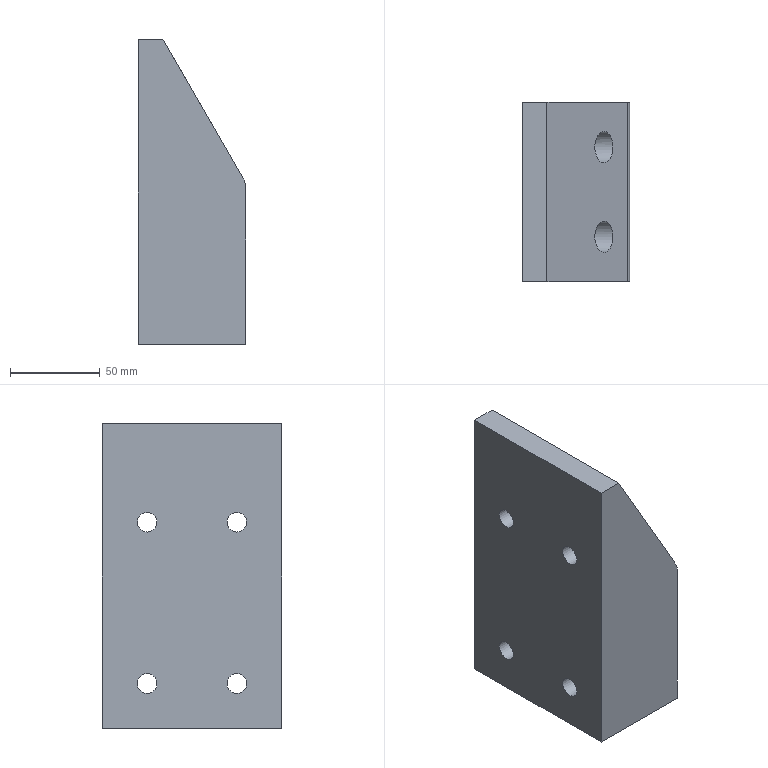Part | NX | features MAIN_BODY 2 | 1 solid | 20 faces | box 60 x 100 x 170 mm | volume 796043 mm3 | plane 11 | cylinder 9 | commonest cylinder face diameters 11 x4 17.5 x4 20 x1
STEP:
#1=CARTESIAN_POINT('',(1053.66,140.,-57.679));
#2=VERTEX_POINT('',#1);
#3=CARTESIAN_POINT('',(1008.812,140.,20.));
#4=VERTEX_POINT('',#3);
#5=CARTESIAN_POINT('',(1094.748,140.,-128.846));
#6=DIRECTION('',(-0.5,0.,0.866));
#7=VECTOR('',#6,1000.);
#8=LINE('',#5,#7);
#9=EDGE_CURVE('',#2,#4,#8,.T.);
#10=ORIENTED_EDGE('',*,*,#9,.T.);
#11=CARTESIAN_POINT('',(995.,140.,20.));
#12=VERTEX_POINT('',#11);
#13=CARTESIAN_POINT('',(850.,140.,20.));
#14=DIRECTION('',(-1.,0.,0.));
#15=VECTOR('',#14,1000.);
#16=LINE('',#13,#15);
#17=EDGE_CURVE('',#4,#12,#16,.T.);
#18=ORIENTED_EDGE('',*,*,#17,.T.);
#19=CARTESIAN_POINT('',(995.,140.,-150.));
#20=VERTEX_POINT('',#19);
#21=CARTESIAN_POINT('',(995.,140.,-335.));
#22=DIRECTION('',(0.,0.,1.));
#23=VECTOR('',#22,1000.);
#24=LINE('',#21,#23);
#25=EDGE_CURVE('',#20,#12,#24,.T.);
#26=ORIENTED_EDGE('',*,*,#25,.F.);
#27=CARTESIAN_POINT('',(1055.,140.,-150.));
#28=VERTEX_POINT('',#27);
#29=CARTESIAN_POINT('',(906.301,140.,-150.));
#30=DIRECTION('',(1.,0.,0.));
#31=VECTOR('',#30,1000.);
#32=LINE('',#29,#31);
#33=EDGE_CURVE('',#20,#28,#32,.T.);
#34=ORIENTED_EDGE('',*,*,#33,.T.);
#35=CARTESIAN_POINT('',(1055.,140.,-62.679));
#36=VERTEX_POINT('',#35);
#37=CARTESIAN_POINT('',(1055.,140.,-335.));
#38=DIRECTION('',(0.,0.,-1.));
#39=VECTOR('',#38,1000.);
#40=LINE('',#37,#39);
#41=EDGE_CURVE('',#36,#28,#40,.T.);
#42=ORIENTED_EDGE('',*,*,#41,.F.);
#43=CARTESIAN_POINT('',(1045.,140.,-62.679));
#44=DIRECTION('',(0.,-1.,0.));
#45=DIRECTION('',(1.,0.,0.));
#46=AXIS2_PLACEMENT_3D('',#43,#44,#45);
#47=CIRCLE('',#46,10.);
#48=EDGE_CURVE('',#2,#36,#47,.F.);
#49=ORIENTED_EDGE('',*,*,#48,.F.);
#50=EDGE_LOOP('',(#10,#18,#26,#34,#42,#49));
#51=FACE_BOUND('',#50,.T.);
#52=CARTESIAN_POINT('',(865.,140.,-335.));
#53=DIRECTION('',(0.,1.,0.));
#54=DIRECTION('',(0.,0.,1.));
#55=AXIS2_PLACEMENT_3D('',#52,#53,#54);
#56=PLANE('',#55);
#57=ADVANCED_FACE('',(#51),#56,.F.);
#58=CARTESIAN_POINT('',(1055.,240.,-150.));
#59=VERTEX_POINT('',#58);
#60=CARTESIAN_POINT('',(1055.,240.,-62.679));
#61=VERTEX_POINT('',#60);
#62=CARTESIAN_POINT('',(1055.,240.,-335.));
#63=DIRECTION('',(0.,0.,-1.));
#64=VECTOR('',#63,1000.);
#65=LINE('',#62,#64);
#66=EDGE_CURVE('',#59,#61,#65,.F.);
#67=ORIENTED_EDGE('',*,*,#66,.F.);
#68=CARTESIAN_POINT('',(995.,240.,-150.));
#69=VERTEX_POINT('',#68);
#70=CARTESIAN_POINT('',(906.301,240.,-150.));
#71=DIRECTION('',(1.,0.,0.));
#72=VECTOR('',#71,1000.);
#73=LINE('',#70,#72);
#74=EDGE_CURVE('',#59,#69,#73,.F.);
#75=ORIENTED_EDGE('',*,*,#74,.T.);
#76=CARTESIAN_POINT('',(995.,240.,20.));
#77=VERTEX_POINT('',#76);
#78=CARTESIAN_POINT('',(995.,240.,-335.));
#79=DIRECTION('',(0.,0.,-1.));
#80=VECTOR('',#79,1000.);
#81=LINE('',#78,#80);
#82=EDGE_CURVE('',#69,#77,#81,.F.);
#83=ORIENTED_EDGE('',*,*,#82,.T.);
#84=CARTESIAN_POINT('',(1008.812,240.,20.));
#85=VERTEX_POINT('',#84);
#86=CARTESIAN_POINT('',(850.,240.,20.));
#87=DIRECTION('',(-1.,0.,0.));
#88=VECTOR('',#87,1000.);
#89=LINE('',#86,#88);
#90=EDGE_CURVE('',#77,#85,#89,.F.);
#91=ORIENTED_EDGE('',*,*,#90,.T.);
#92=CARTESIAN_POINT('',(1053.66,240.,-57.679));
#93=VERTEX_POINT('',#92);
#94=CARTESIAN_POINT('',(1094.748,240.,-128.846));
#95=DIRECTION('',(-0.5,0.,0.866));
#96=VECTOR('',#95,1000.);
#97=LINE('',#94,#96);
#98=EDGE_CURVE('',#93,#85,#97,.T.);
#99=ORIENTED_EDGE('',*,*,#98,.F.);
#100=CARTESIAN_POINT('',(1045.,240.,-62.679));
#101=DIRECTION('',(0.,-1.,0.));
#102=DIRECTION('',(1.,0.,0.));
#103=AXIS2_PLACEMENT_3D('',#100,#101,#102);
#104=CIRCLE('',#103,10.);
#105=EDGE_CURVE('',#61,#93,#104,.T.);
#106=ORIENTED_EDGE('',*,*,#105,.F.);
#107=EDGE_LOOP('',(#67,#75,#83,#91,#99,#106));
#108=FACE_BOUND('',#107,.T.);
#109=CARTESIAN_POINT('',(865.,240.,-335.));
#110=DIRECTION('',(0.,1.,0.));
#111=DIRECTION('',(0.,0.,1.));
#112=AXIS2_PLACEMENT_3D('',#109,#110,#111);
#113=PLANE('',#112);
#114=ADVANCED_FACE('',(#108),#113,.T.);
#115=CARTESIAN_POINT('',(1055.,223.75,-125.));
#116=VERTEX_POINT('',#115);
#117=CARTESIAN_POINT('',(1055.,215.,-125.));
#118=DIRECTION('',(-1.,0.,0.));
#119=DIRECTION('',(0.,1.,0.));
#120=AXIS2_PLACEMENT_3D('',#117,#118,#119);
#121=CIRCLE('',#120,8.75);
#122=EDGE_CURVE('',#116,#116,#121,.T.);
#123=ORIENTED_EDGE('',*,*,#122,.T.);
#124=EDGE_LOOP('',(#123));
#125=FACE_BOUND('',#124,.T.);
#126=CARTESIAN_POINT('',(1055.,173.75,-125.));
#127=VERTEX_POINT('',#126);
#128=CARTESIAN_POINT('',(1055.,165.,-125.));
#129=DIRECTION('',(-1.,0.,0.));
#130=DIRECTION('',(0.,1.,0.));
#131=AXIS2_PLACEMENT_3D('',#128,#129,#130);
#132=CIRCLE('',#131,8.75);
#133=EDGE_CURVE('',#127,#127,#132,.T.);
#134=ORIENTED_EDGE('',*,*,#133,.T.);
#135=EDGE_LOOP('',(#134));
#136=FACE_BOUND('',#135,.T.);
#137=ORIENTED_EDGE('',*,*,#41,.T.);
#138=CARTESIAN_POINT('',(1055.,114.375,-150.));
#139=DIRECTION('',(0.,1.,0.));
#140=VECTOR('',#139,1000.);
#141=LINE('',#138,#140);
#142=EDGE_CURVE('',#28,#59,#141,.T.);
#143=ORIENTED_EDGE('',*,*,#142,.T.);
#144=ORIENTED_EDGE('',*,*,#66,.T.);
#145=CARTESIAN_POINT('',(1055.,230.,-62.679));
#146=DIRECTION('',(0.,-1.,0.));
#147=VECTOR('',#146,1000.);
#148=LINE('',#145,#147);
#149=EDGE_CURVE('',#36,#61,#148,.F.);
#150=ORIENTED_EDGE('',*,*,#149,.F.);
#151=EDGE_LOOP('',(#137,#143,#144,#150));
#152=FACE_BOUND('',#151,.T.);
#153=CARTESIAN_POINT('',(1055.,190.,-105.));
#154=DIRECTION('',(-1.,0.,0.));
#155=DIRECTION('',(0.,-1.,0.));
#156=AXIS2_PLACEMENT_3D('',#153,#154,#155);
#157=PLANE('',#156);
#158=ADVANCED_FACE('',(#125,#136,#152),#157,.F.);
#159=CARTESIAN_POINT('',(1015.,165.,-26.25));
#160=VERTEX_POINT('',#159);
#161=CARTESIAN_POINT('',(1015.,165.,-35.));
#162=DIRECTION('',(-1.,0.,0.));
#163=DIRECTION('',(0.,0.,1.));
#164=AXIS2_PLACEMENT_3D('',#161,#162,#163);
#165=CIRCLE('',#164,8.75);
#166=EDGE_CURVE('',#160,#160,#165,.T.);
#167=ORIENTED_EDGE('',*,*,#166,.T.);
#168=EDGE_LOOP('',(#167));
#169=FACE_BOUND('',#168,.T.);
#170=CARTESIAN_POINT('',(1045.618,165.,-43.75));
#171=VERTEX_POINT('',#170);
#172=CARTESIAN_POINT('',(1040.566,165.,-35.));
#173=DIRECTION('',(-0.866,0.,-0.5));
#174=DIRECTION('',(0.5,0.,-0.866));
#175=AXIS2_PLACEMENT_3D('',#172,#173,#174);
#176=ELLIPSE('',#175,10.104,8.75);
#177=EDGE_CURVE('',#171,#171,#176,.F.);
#178=ORIENTED_EDGE('',*,*,#177,.T.);
#179=EDGE_LOOP('',(#178));
#180=FACE_BOUND('',#179,.T.);
#181=CARTESIAN_POINT('',(1020.,165.,-35.));
#182=DIRECTION('',(1.,0.,0.));
#183=DIRECTION('',(0.,0.,1.));
#184=AXIS2_PLACEMENT_3D('',#181,#182,#183);
#185=CYLINDRICAL_SURFACE('',#184,8.75);
#186=ADVANCED_FACE('',(#169,#180),#185,.F.);
#187=CARTESIAN_POINT('',(1015.,215.,-26.25));
#188=VERTEX_POINT('',#187);
#189=CARTESIAN_POINT('',(1015.,215.,-35.));
#190=DIRECTION('',(-1.,0.,0.));
#191=DIRECTION('',(0.,0.,1.));
#192=AXIS2_PLACEMENT_3D('',#189,#190,#191);
#193=CIRCLE('',#192,8.75);
#194=EDGE_CURVE('',#188,#188,#193,.T.);
#195=ORIENTED_EDGE('',*,*,#194,.T.);
#196=EDGE_LOOP('',(#195));
#197=FACE_BOUND('',#196,.T.);
#198=CARTESIAN_POINT('',(1045.618,215.,-43.75));
#199=VERTEX_POINT('',#198);
#200=CARTESIAN_POINT('',(1040.566,215.,-35.));
#201=DIRECTION('',(-0.866,0.,-0.5));
#202=DIRECTION('',(0.5,0.,-0.866));
#203=AXIS2_PLACEMENT_3D('',#200,#201,#202);
#204=ELLIPSE('',#203,10.104,8.75);
#205=EDGE_CURVE('',#199,#199,#204,.F.);
#206=ORIENTED_EDGE('',*,*,#205,.T.);
#207=EDGE_LOOP('',(#206));
#208=FACE_BOUND('',#207,.T.);
#209=CARTESIAN_POINT('',(1020.,215.,-35.));
#210=DIRECTION('',(1.,0.,0.));
#211=DIRECTION('',(0.,0.,1.));
#212=AXIS2_PLACEMENT_3D('',#209,#210,#211);
#213=CYLINDRICAL_SURFACE('',#212,8.75);
#214=ADVANCED_FACE('',(#197,#208),#213,.F.);
#215=CARTESIAN_POINT('',(995.,165.,-29.5));
#216=VERTEX_POINT('',#215);
#217=CARTESIAN_POINT('',(995.,165.,-35.));
#218=DIRECTION('',(-1.,0.,0.));
#219=DIRECTION('',(0.,0.,1.));
#220=AXIS2_PLACEMENT_3D('',#217,#218,#219);
#221=CIRCLE('',#220,5.5);
#222=EDGE_CURVE('',#216,#216,#221,.F.);
#223=ORIENTED_EDGE('',*,*,#222,.T.);
#224=EDGE_LOOP('',(#223));
#225=FACE_BOUND('',#224,.T.);
#226=CARTESIAN_POINT('',(995.,165.,-119.5));
#227=VERTEX_POINT('',#226);
#228=CARTESIAN_POINT('',(995.,165.,-125.));
#229=DIRECTION('',(-1.,0.,0.));
#230=DIRECTION('',(0.,0.,1.));
#231=AXIS2_PLACEMENT_3D('',#228,#229,#230);
#232=CIRCLE('',#231,5.5);
#233=EDGE_CURVE('',#227,#227,#232,.F.);
#234=ORIENTED_EDGE('',*,*,#233,.T.);
#235=EDGE_LOOP('',(#234));
#236=FACE_BOUND('',#235,.T.);
#237=CARTESIAN_POINT('',(995.,215.,-119.5));
#238=VERTEX_POINT('',#237);
#239=CARTESIAN_POINT('',(995.,215.,-125.));
#240=DIRECTION('',(-1.,0.,0.));
#241=DIRECTION('',(0.,0.,1.));
#242=AXIS2_PLACEMENT_3D('',#239,#240,#241);
#243=CIRCLE('',#242,5.5);
#244=EDGE_CURVE('',#238,#238,#243,.F.);
#245=ORIENTED_EDGE('',*,*,#244,.T.);
#246=EDGE_LOOP('',(#245));
#247=FACE_BOUND('',#246,.T.);
#248=ORIENTED_EDGE('',*,*,#82,.F.);
#249=CARTESIAN_POINT('',(995.,114.375,-150.));
#250=DIRECTION('',(0.,-1.,0.));
#251=VECTOR('',#250,1000.);
#252=LINE('',#249,#251);
#253=EDGE_CURVE('',#69,#20,#252,.T.);
#254=ORIENTED_EDGE('',*,*,#253,.T.);
#255=ORIENTED_EDGE('',*,*,#25,.T.);
#256=CARTESIAN_POINT('',(995.,195.,20.));
#257=DIRECTION('',(0.,1.,0.));
#258=VECTOR('',#257,1000.);
#259=LINE('',#256,#258);
#260=EDGE_CURVE('',#12,#77,#259,.T.);
#261=ORIENTED_EDGE('',*,*,#260,.T.);
#262=EDGE_LOOP('',(#248,#254,#255,#261));
#263=FACE_BOUND('',#262,.T.);
#264=CARTESIAN_POINT('',(995.,215.,-29.5));
#265=VERTEX_POINT('',#264);
#266=CARTESIAN_POINT('',(995.,215.,-35.));
#267=DIRECTION('',(-1.,0.,0.));
#268=DIRECTION('',(0.,0.,1.));
#269=AXIS2_PLACEMENT_3D('',#266,#267,#268);
#270=CIRCLE('',#269,5.5);
#271=EDGE_CURVE('',#265,#265,#270,.F.);
#272=ORIENTED_EDGE('',*,*,#271,.T.);
#273=EDGE_LOOP('',(#272));
#274=FACE_BOUND('',#273,.T.);
#275=CARTESIAN_POINT('',(995.,95.,-335.));
#276=DIRECTION('',(1.,0.,0.));
#277=DIRECTION('',(0.,1.,0.));
#278=AXIS2_PLACEMENT_3D('',#275,#276,#277);
#279=PLANE('',#278);
#280=ADVANCED_FACE('',(#225,#236,#247,#263,#274),#279,.F.);
#281=ORIENTED_EDGE('',*,*,#90,.F.);
#282=ORIENTED_EDGE('',*,*,#260,.F.);
#283=ORIENTED_EDGE('',*,*,#17,.F.);
#284=CARTESIAN_POINT('',(1008.812,195.,20.));
#285=DIRECTION('',(0.,1.,0.));
#286=VECTOR('',#285,1000.);
#287=LINE('',#284,#286);
#288=EDGE_CURVE('',#4,#85,#287,.T.);
#289=ORIENTED_EDGE('',*,*,#288,.T.);
#290=EDGE_LOOP('',(#281,#282,#283,#289));
#291=FACE_BOUND('',#290,.T.);
#292=CARTESIAN_POINT('',(850.,195.,20.));
#293=DIRECTION('',(0.,0.,-1.));
#294=DIRECTION('',(0.4226,0.9063,0.));
#295=AXIS2_PLACEMENT_3D('',#292,#293,#294);
#296=PLANE('',#295);
#297=ADVANCED_FACE('',(#291),#296,.F.);
#298=ORIENTED_EDGE('',*,*,#33,.F.);
#299=ORIENTED_EDGE('',*,*,#253,.F.);
#300=ORIENTED_EDGE('',*,*,#74,.F.);
#301=ORIENTED_EDGE('',*,*,#142,.F.);
#302=EDGE_LOOP('',(#298,#299,#300,#301));
#303=FACE_BOUND('',#302,.T.);
#304=CARTESIAN_POINT('',(906.301,114.375,-150.));
#305=DIRECTION('',(0.,0.,1.));
#306=DIRECTION('',(0.866,-0.5,0.));
#307=AXIS2_PLACEMENT_3D('',#304,#305,#306);
#308=PLANE('',#307);
#309=ADVANCED_FACE('',(#303),#308,.F.);
#310=CARTESIAN_POINT('',(1015.,215.,-130.5));
#311=VERTEX_POINT('',#310);
#312=CARTESIAN_POINT('',(1015.,215.,-125.));
#313=DIRECTION('',(1.,0.,0.));
#314=DIRECTION('',(0.,0.,-1.));
#315=AXIS2_PLACEMENT_3D('',#312,#313,#314);
#316=CIRCLE('',#315,5.5);
#317=EDGE_CURVE('',#311,#311,#316,.F.);
#318=ORIENTED_EDGE('',*,*,#317,.F.);
#319=EDGE_LOOP('',(#318));
#320=FACE_BOUND('',#319,.T.);
#321=ORIENTED_EDGE('',*,*,#244,.F.);
#322=EDGE_LOOP('',(#321));
#323=FACE_BOUND('',#322,.T.);
#324=CARTESIAN_POINT('',(875.,215.,-125.));
#325=DIRECTION('',(-1.,0.,0.));
#326=DIRECTION('',(0.,1.,0.));
#327=AXIS2_PLACEMENT_3D('',#324,#325,#326);
#328=CYLINDRICAL_SURFACE('',#327,5.5);
#329=ADVANCED_FACE('',(#320,#323),#328,.F.);
#330=ORIENTED_EDGE('',*,*,#317,.T.);
#331=EDGE_LOOP('',(#330));
#332=FACE_BOUND('',#331,.T.);
#333=CARTESIAN_POINT('',(1015.,215.,-133.75));
#334=VERTEX_POINT('',#333);
#335=CARTESIAN_POINT('',(1015.,215.,-125.));
#336=DIRECTION('',(1.,0.,0.));
#337=DIRECTION('',(0.,0.,-1.));
#338=AXIS2_PLACEMENT_3D('',#335,#336,#337);
#339=CIRCLE('',#338,8.75);
#340=EDGE_CURVE('',#334,#334,#339,.F.);
#341=ORIENTED_EDGE('',*,*,#340,.F.);
#342=EDGE_LOOP('',(#341));
#343=FACE_BOUND('',#342,.T.);
#344=CARTESIAN_POINT('',(1015.,195.,-75.));
#345=DIRECTION('',(-1.,0.,0.));
#346=DIRECTION('',(0.,1.,0.));
#347=AXIS2_PLACEMENT_3D('',#344,#345,#346);
#348=PLANE('',#347);
#349=ADVANCED_FACE('',(#332,#343),#348,.F.);
#350=ORIENTED_EDGE('',*,*,#340,.T.);
#351=EDGE_LOOP('',(#350));
#352=FACE_BOUND('',#351,.T.);
#353=ORIENTED_EDGE('',*,*,#122,.F.);
#354=EDGE_LOOP('',(#353));
#355=FACE_BOUND('',#354,.T.);
#356=CARTESIAN_POINT('',(1075.,215.,-125.));
#357=DIRECTION('',(-1.,0.,0.));
#358=DIRECTION('',(0.,1.,0.));
#359=AXIS2_PLACEMENT_3D('',#356,#357,#358);
#360=CYLINDRICAL_SURFACE('',#359,8.75);
#361=ADVANCED_FACE('',(#352,#355),#360,.F.);
#362=CARTESIAN_POINT('',(1015.,165.,-130.5));
#363=VERTEX_POINT('',#362);
#364=CARTESIAN_POINT('',(1015.,165.,-125.));
#365=DIRECTION('',(1.,0.,0.));
#366=DIRECTION('',(0.,0.,-1.));
#367=AXIS2_PLACEMENT_3D('',#364,#365,#366);
#368=CIRCLE('',#367,5.5);
#369=EDGE_CURVE('',#363,#363,#368,.F.);
#370=ORIENTED_EDGE('',*,*,#369,.F.);
#371=EDGE_LOOP('',(#370));
#372=FACE_BOUND('',#371,.T.);
#373=ORIENTED_EDGE('',*,*,#233,.F.);
#374=EDGE_LOOP('',(#373));
#375=FACE_BOUND('',#374,.T.);
#376=CARTESIAN_POINT('',(875.,165.,-125.));
#377=DIRECTION('',(-1.,0.,0.));
#378=DIRECTION('',(0.,1.,0.));
#379=AXIS2_PLACEMENT_3D('',#376,#377,#378);
#380=CYLINDRICAL_SURFACE('',#379,5.5);
#381=ADVANCED_FACE('',(#372,#375),#380,.F.);
#382=ORIENTED_EDGE('',*,*,#369,.T.);
#383=EDGE_LOOP('',(#382));
#384=FACE_BOUND('',#383,.T.);
#385=CARTESIAN_POINT('',(1015.,165.,-133.75));
#386=VERTEX_POINT('',#385);
#387=CARTESIAN_POINT('',(1015.,165.,-125.));
#388=DIRECTION('',(1.,0.,0.));
#389=DIRECTION('',(0.,0.,-1.));
#390=AXIS2_PLACEMENT_3D('',#387,#388,#389);
#391=CIRCLE('',#390,8.75);
#392=EDGE_CURVE('',#386,#386,#391,.F.);
#393=ORIENTED_EDGE('',*,*,#392,.F.);
#394=EDGE_LOOP('',(#393));
#395=FACE_BOUND('',#394,.T.);
#396=CARTESIAN_POINT('',(1015.,110.,-75.));
#397=DIRECTION('',(-1.,0.,0.));
#398=DIRECTION('',(0.,1.,0.));
#399=AXIS2_PLACEMENT_3D('',#396,#397,#398);
#400=PLANE('',#399);
#401=ADVANCED_FACE('',(#384,#395),#400,.F.);
#402=ORIENTED_EDGE('',*,*,#392,.T.);
#403=EDGE_LOOP('',(#402));
#404=FACE_BOUND('',#403,.T.);
#405=ORIENTED_EDGE('',*,*,#133,.F.);
#406=EDGE_LOOP('',(#405));
#407=FACE_BOUND('',#406,.T.);
#408=CARTESIAN_POINT('',(1075.,165.,-125.));
#409=DIRECTION('',(-1.,0.,0.));
#410=DIRECTION('',(0.,1.,0.));
#411=AXIS2_PLACEMENT_3D('',#408,#409,#410);
#412=CYLINDRICAL_SURFACE('',#411,8.75);
#413=ADVANCED_FACE('',(#404,#407),#412,.F.);
#414=ORIENTED_EDGE('',*,*,#222,.F.);
#415=EDGE_LOOP('',(#414));
#416=FACE_BOUND('',#415,.T.);
#417=CARTESIAN_POINT('',(1015.,165.,-29.5));
#418=VERTEX_POINT('',#417);
#419=CARTESIAN_POINT('',(1015.,165.,-35.));
#420=DIRECTION('',(-1.,0.,0.));
#421=DIRECTION('',(0.,0.,1.));
#422=AXIS2_PLACEMENT_3D('',#419,#420,#421);
#423=CIRCLE('',#422,5.5);
#424=EDGE_CURVE('',#418,#418,#423,.T.);
#425=ORIENTED_EDGE('',*,*,#424,.F.);
#426=EDGE_LOOP('',(#425));
#427=FACE_BOUND('',#426,.T.);
#428=CARTESIAN_POINT('',(995.,165.,-35.));
#429=DIRECTION('',(1.,0.,0.));
#430=DIRECTION('',(0.,0.,1.));
#431=AXIS2_PLACEMENT_3D('',#428,#429,#430);
#432=CYLINDRICAL_SURFACE('',#431,5.5);
#433=ADVANCED_FACE('',(#416,#427),#432,.F.);
#434=ORIENTED_EDGE('',*,*,#166,.F.);
#435=EDGE_LOOP('',(#434));
#436=FACE_BOUND('',#435,.T.);
#437=ORIENTED_EDGE('',*,*,#424,.T.);
#438=EDGE_LOOP('',(#437));
#439=FACE_BOUND('',#438,.T.);
#440=CARTESIAN_POINT('',(1015.,140.,-50.));
#441=DIRECTION('',(1.,0.,0.));
#442=DIRECTION('',(0.,0.,1.));
#443=AXIS2_PLACEMENT_3D('',#440,#441,#442);
#444=PLANE('',#443);
#445=ADVANCED_FACE('',(#436,#439),#444,.T.);
#446=ORIENTED_EDGE('',*,*,#271,.F.);
#447=EDGE_LOOP('',(#446));
#448=FACE_BOUND('',#447,.T.);
#449=CARTESIAN_POINT('',(1015.,215.,-29.5));
#450=VERTEX_POINT('',#449);
#451=CARTESIAN_POINT('',(1015.,215.,-35.));
#452=DIRECTION('',(-1.,0.,0.));
#453=DIRECTION('',(0.,0.,1.));
#454=AXIS2_PLACEMENT_3D('',#451,#452,#453);
#455=CIRCLE('',#454,5.5);
#456=EDGE_CURVE('',#450,#450,#455,.T.);
#457=ORIENTED_EDGE('',*,*,#456,.F.);
#458=EDGE_LOOP('',(#457));
#459=FACE_BOUND('',#458,.T.);
#460=CARTESIAN_POINT('',(995.,215.,-35.));
#461=DIRECTION('',(1.,0.,0.));
#462=DIRECTION('',(0.,0.,1.));
#463=AXIS2_PLACEMENT_3D('',#460,#461,#462);
#464=CYLINDRICAL_SURFACE('',#463,5.5);
#465=ADVANCED_FACE('',(#448,#459),#464,.F.);
#466=ORIENTED_EDGE('',*,*,#194,.F.);
#467=EDGE_LOOP('',(#466));
#468=FACE_BOUND('',#467,.T.);
#469=ORIENTED_EDGE('',*,*,#456,.T.);
#470=EDGE_LOOP('',(#469));
#471=FACE_BOUND('',#470,.T.);
#472=CARTESIAN_POINT('',(1015.,195.,-50.));
#473=DIRECTION('',(1.,0.,0.));
#474=DIRECTION('',(0.,0.,1.));
#475=AXIS2_PLACEMENT_3D('',#472,#473,#474);
#476=PLANE('',#475);
#477=ADVANCED_FACE('',(#468,#471),#476,.T.);
#478=ORIENTED_EDGE('',*,*,#205,.F.);
#479=EDGE_LOOP('',(#478));
#480=FACE_BOUND('',#479,.T.);
#481=ORIENTED_EDGE('',*,*,#177,.F.);
#482=EDGE_LOOP('',(#481));
#483=FACE_BOUND('',#482,.T.);
#484=ORIENTED_EDGE('',*,*,#98,.T.);
#485=ORIENTED_EDGE('',*,*,#288,.F.);
#486=ORIENTED_EDGE('',*,*,#9,.F.);
#487=CARTESIAN_POINT('',(1053.66,130.,-57.679));
#488=DIRECTION('',(0.,-1.,0.));
#489=VECTOR('',#488,1000.);
#490=LINE('',#487,#489);
#491=EDGE_CURVE('',#93,#2,#490,.T.);
#492=ORIENTED_EDGE('',*,*,#491,.F.);
#493=EDGE_LOOP('',(#484,#485,#486,#492));
#494=FACE_BOUND('',#493,.T.);
#495=CARTESIAN_POINT('',(1094.748,230.,-128.846));
#496=DIRECTION('',(0.866,0.,0.5));
#497=DIRECTION('',(0.5,0.,-0.866));
#498=AXIS2_PLACEMENT_3D('',#495,#496,#497);
#499=PLANE('',#498);
#500=ADVANCED_FACE('',(#480,#483,#494),#499,.T.);
#501=ORIENTED_EDGE('',*,*,#105,.T.);
#502=ORIENTED_EDGE('',*,*,#491,.T.);
#503=ORIENTED_EDGE('',*,*,#48,.T.);
#504=ORIENTED_EDGE('',*,*,#149,.T.);
#505=EDGE_LOOP('',(#501,#502,#503,#504));
#506=FACE_BOUND('',#505,.T.);
#507=CARTESIAN_POINT('',(1045.,230.,-62.679));
#508=DIRECTION('',(0.,1.,0.));
#509=DIRECTION('',(1.,0.,0.));
#510=AXIS2_PLACEMENT_3D('',#507,#508,#509);
#511=CYLINDRICAL_SURFACE('',#510,10.);
#512=ADVANCED_FACE('',(#506),#511,.T.);
#513=CLOSED_SHELL('',(#57,#114,#158,#186,#214,#280,#297,#309,#329,#349,#361,#381,#401,#413,#433,#445,#465,#477,#500,#512));
#514=MANIFOLD_SOLID_BREP('',#513);
#515=(LENGTH_UNIT()NAMED_UNIT(*)SI_UNIT(.MILLI.,.METRE.));
#516=UNCERTAINTY_MEASURE_WITH_UNIT(LENGTH_MEASURE(0.00001),#515,'','');
#517=(NAMED_UNIT(*)PLANE_ANGLE_UNIT()SI_UNIT($,.RADIAN.));
#518=(NAMED_UNIT(*)SI_UNIT($,.STERADIAN.)SOLID_ANGLE_UNIT());
#519=(GEOMETRIC_REPRESENTATION_CONTEXT(3)GLOBAL_UNCERTAINTY_ASSIGNED_CONTEXT((#516))GLOBAL_UNIT_ASSIGNED_CONTEXT((#515,#517,#518))REPRESENTATION_CONTEXT('',''));
#520=ADVANCED_BREP_SHAPE_REPRESENTATION('',(#514),#519);